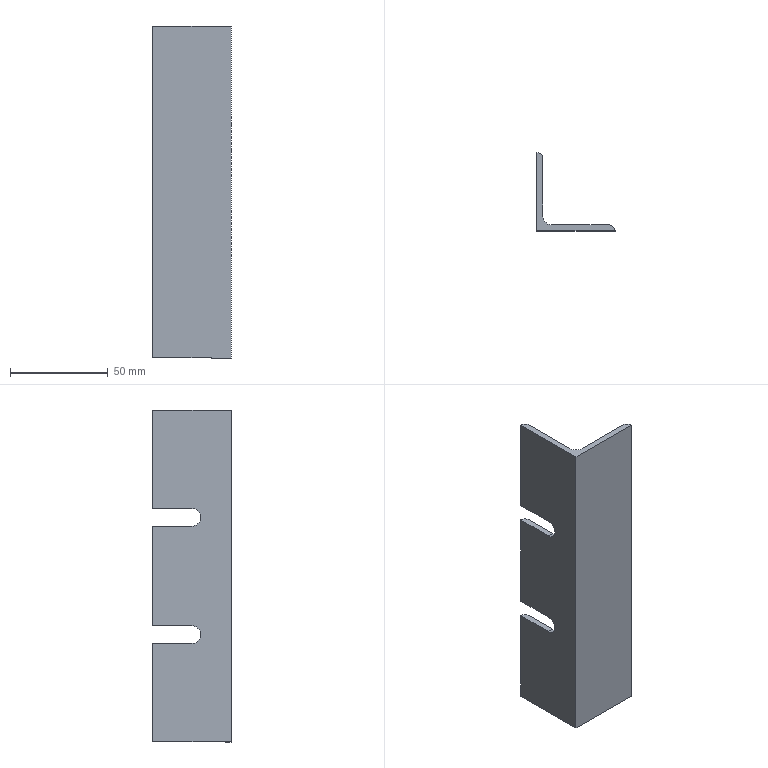Part | SolidWorks | features BaseBody 1 | 1 solid | 17 faces | box 40 x 40 x 170 mm | volume 38116 mm3 | plane 10 | cylinder 7 | commonest cylinder face diameters 6 x4 9 x3
STEP:
#1=CARTESIAN_POINT('',(3.,37.,25.5));
#2=VERTEX_POINT('',#1);
#3=CARTESIAN_POINT('',(0.,40.,25.5));
#4=VERTEX_POINT('',#3);
#5=CARTESIAN_POINT('',(0.,37.,25.5));
#6=DIRECTION('',(0.,0.,1.));
#7=DIRECTION('',(0.,1.,0.));
#8=AXIS2_PLACEMENT_3D('',#5,#6,#7);
#9=CIRCLE('',#8,3.);
#10=EDGE_CURVE('',#2,#4,#9,.T.);
#11=ORIENTED_EDGE('',*,*,#10,.T.);
#12=CARTESIAN_POINT('',(0.,20.,25.5));
#13=VERTEX_POINT('',#12);
#14=CARTESIAN_POINT('',(0.,40.,25.5));
#15=DIRECTION('',(0.,-1.,0.));
#16=VECTOR('',#15,1000.);
#17=LINE('',#14,#16);
#18=EDGE_CURVE('',#4,#13,#17,.T.);
#19=ORIENTED_EDGE('',*,*,#18,.T.);
#20=CARTESIAN_POINT('',(3.,20.,25.5));
#21=VERTEX_POINT('',#20);
#22=CARTESIAN_POINT('',(10.,20.,25.5));
#23=DIRECTION('',(-1.,0.,0.));
#24=VECTOR('',#23,1000.);
#25=LINE('',#22,#24);
#26=EDGE_CURVE('',#21,#13,#25,.T.);
#27=ORIENTED_EDGE('',*,*,#26,.F.);
#28=CARTESIAN_POINT('',(3.,40.,25.5));
#29=DIRECTION('',(0.,-1.,0.));
#30=VECTOR('',#29,1000.);
#31=LINE('',#28,#30);
#32=EDGE_CURVE('',#2,#21,#31,.T.);
#33=ORIENTED_EDGE('',*,*,#32,.F.);
#34=EDGE_LOOP('',(#11,#19,#27,#33));
#35=FACE_OUTER_BOUND('',#34,.T.);
#36=CARTESIAN_POINT('',(10.,40.,25.5));
#37=DIRECTION('',(0.,0.,-1.));
#38=DIRECTION('',(0.,-1.,0.));
#39=AXIS2_PLACEMENT_3D('',#36,#37,#38);
#40=PLANE('',#39);
#41=ADVANCED_FACE('',(#35),#40,.F.);
#42=CARTESIAN_POINT('',(3.,20.,34.5));
#43=VERTEX_POINT('',#42);
#44=CARTESIAN_POINT('',(0.,20.,34.5));
#45=VERTEX_POINT('',#44);
#46=CARTESIAN_POINT('',(10.,20.,34.5));
#47=DIRECTION('',(-1.,0.,0.));
#48=VECTOR('',#47,1000.);
#49=LINE('',#46,#48);
#50=EDGE_CURVE('',#43,#45,#49,.T.);
#51=ORIENTED_EDGE('',*,*,#50,.T.);
#52=CARTESIAN_POINT('',(0.,40.,34.5));
#53=VERTEX_POINT('',#52);
#54=CARTESIAN_POINT('',(0.,40.,34.5));
#55=DIRECTION('',(0.,1.,0.));
#56=VECTOR('',#55,1000.);
#57=LINE('',#54,#56);
#58=EDGE_CURVE('',#45,#53,#57,.T.);
#59=ORIENTED_EDGE('',*,*,#58,.T.);
#60=CARTESIAN_POINT('',(3.,37.,34.5));
#61=VERTEX_POINT('',#60);
#62=CARTESIAN_POINT('',(0.,37.,34.5));
#63=DIRECTION('',(0.,0.,-1.));
#64=DIRECTION('',(0.,-1.,0.));
#65=AXIS2_PLACEMENT_3D('',#62,#63,#64);
#66=CIRCLE('',#65,3.);
#67=EDGE_CURVE('',#53,#61,#66,.T.);
#68=ORIENTED_EDGE('',*,*,#67,.T.);
#69=CARTESIAN_POINT('',(3.,40.,34.5));
#70=DIRECTION('',(0.,1.,0.));
#71=VECTOR('',#70,1000.);
#72=LINE('',#69,#71);
#73=EDGE_CURVE('',#43,#61,#72,.T.);
#74=ORIENTED_EDGE('',*,*,#73,.F.);
#75=EDGE_LOOP('',(#51,#59,#68,#74));
#76=FACE_OUTER_BOUND('',#75,.T.);
#77=CARTESIAN_POINT('',(10.,40.,34.5));
#78=DIRECTION('',(0.,0.,1.));
#79=DIRECTION('',(0.,-1.,0.));
#80=AXIS2_PLACEMENT_3D('',#77,#78,#79);
#81=PLANE('',#80);
#82=ADVANCED_FACE('',(#76),#81,.F.);
#83=ORIENTED_EDGE('',*,*,#26,.T.);
#84=CARTESIAN_POINT('',(0.,20.,30.));
#85=DIRECTION('',(-1.,0.,0.));
#86=DIRECTION('',(0.,0.,1.));
#87=AXIS2_PLACEMENT_3D('',#84,#85,#86);
#88=CIRCLE('',#87,4.5);
#89=EDGE_CURVE('',#13,#45,#88,.T.);
#90=ORIENTED_EDGE('',*,*,#89,.T.);
#91=ORIENTED_EDGE('',*,*,#50,.F.);
#92=CARTESIAN_POINT('',(3.,20.,30.));
#93=DIRECTION('',(-1.,0.,0.));
#94=DIRECTION('',(0.,-1.,0.));
#95=AXIS2_PLACEMENT_3D('',#92,#93,#94);
#96=CIRCLE('',#95,4.5);
#97=EDGE_CURVE('',#21,#43,#96,.T.);
#98=ORIENTED_EDGE('',*,*,#97,.F.);
#99=EDGE_LOOP('',(#83,#90,#91,#98));
#100=FACE_OUTER_BOUND('',#99,.T.);
#101=CARTESIAN_POINT('',(10.,20.,30.));
#102=DIRECTION('',(-1.,0.,0.));
#103=DIRECTION('',(0.,0.,1.));
#104=AXIS2_PLACEMENT_3D('',#101,#102,#103);
#105=CYLINDRICAL_SURFACE('',#104,4.5);
#106=ADVANCED_FACE('',(#100),#105,.F.);
#107=CARTESIAN_POINT('',(3.,37.,-34.5));
#108=VERTEX_POINT('',#107);
#109=CARTESIAN_POINT('',(0.,40.,-34.5));
#110=VERTEX_POINT('',#109);
#111=CARTESIAN_POINT('',(0.,37.,-34.5));
#112=DIRECTION('',(0.,0.,1.));
#113=DIRECTION('',(0.,1.,0.));
#114=AXIS2_PLACEMENT_3D('',#111,#112,#113);
#115=CIRCLE('',#114,3.);
#116=EDGE_CURVE('',#108,#110,#115,.T.);
#117=ORIENTED_EDGE('',*,*,#116,.T.);
#118=CARTESIAN_POINT('',(0.,20.,-34.5));
#119=VERTEX_POINT('',#118);
#120=CARTESIAN_POINT('',(0.,40.,-34.5));
#121=DIRECTION('',(0.,-1.,0.));
#122=VECTOR('',#121,1000.);
#123=LINE('',#120,#122);
#124=EDGE_CURVE('',#110,#119,#123,.T.);
#125=ORIENTED_EDGE('',*,*,#124,.T.);
#126=CARTESIAN_POINT('',(3.,20.,-34.5));
#127=VERTEX_POINT('',#126);
#128=CARTESIAN_POINT('',(10.,20.,-34.5));
#129=DIRECTION('',(-1.,0.,0.));
#130=VECTOR('',#129,1000.);
#131=LINE('',#128,#130);
#132=EDGE_CURVE('',#127,#119,#131,.T.);
#133=ORIENTED_EDGE('',*,*,#132,.F.);
#134=CARTESIAN_POINT('',(3.,40.,-34.5));
#135=DIRECTION('',(0.,-1.,0.));
#136=VECTOR('',#135,1000.);
#137=LINE('',#134,#136);
#138=EDGE_CURVE('',#108,#127,#137,.T.);
#139=ORIENTED_EDGE('',*,*,#138,.F.);
#140=EDGE_LOOP('',(#117,#125,#133,#139));
#141=FACE_OUTER_BOUND('',#140,.T.);
#142=CARTESIAN_POINT('',(10.,40.,-34.5));
#143=DIRECTION('',(0.,0.,-1.));
#144=DIRECTION('',(0.,-1.,0.));
#145=AXIS2_PLACEMENT_3D('',#142,#143,#144);
#146=PLANE('',#145);
#147=ADVANCED_FACE('',(#141),#146,.F.);
#148=CARTESIAN_POINT('',(3.,20.,-25.5));
#149=VERTEX_POINT('',#148);
#150=CARTESIAN_POINT('',(0.,20.,-25.5));
#151=VERTEX_POINT('',#150);
#152=CARTESIAN_POINT('',(10.,20.,-25.5));
#153=DIRECTION('',(-1.,0.,0.));
#154=VECTOR('',#153,1000.);
#155=LINE('',#152,#154);
#156=EDGE_CURVE('',#149,#151,#155,.T.);
#157=ORIENTED_EDGE('',*,*,#156,.T.);
#158=CARTESIAN_POINT('',(0.,40.,-25.5));
#159=VERTEX_POINT('',#158);
#160=CARTESIAN_POINT('',(0.,40.,-25.5));
#161=DIRECTION('',(0.,1.,0.));
#162=VECTOR('',#161,1000.);
#163=LINE('',#160,#162);
#164=EDGE_CURVE('',#151,#159,#163,.T.);
#165=ORIENTED_EDGE('',*,*,#164,.T.);
#166=CARTESIAN_POINT('',(3.,37.,-25.5));
#167=VERTEX_POINT('',#166);
#168=CARTESIAN_POINT('',(0.,37.,-25.5));
#169=DIRECTION('',(0.,0.,-1.));
#170=DIRECTION('',(1.,0.,0.));
#171=AXIS2_PLACEMENT_3D('',#168,#169,#170);
#172=CIRCLE('',#171,3.);
#173=EDGE_CURVE('',#159,#167,#172,.T.);
#174=ORIENTED_EDGE('',*,*,#173,.T.);
#175=CARTESIAN_POINT('',(3.,40.,-25.5));
#176=DIRECTION('',(0.,1.,0.));
#177=VECTOR('',#176,1000.);
#178=LINE('',#175,#177);
#179=EDGE_CURVE('',#149,#167,#178,.T.);
#180=ORIENTED_EDGE('',*,*,#179,.F.);
#181=EDGE_LOOP('',(#157,#165,#174,#180));
#182=FACE_OUTER_BOUND('',#181,.T.);
#183=CARTESIAN_POINT('',(10.,40.,-25.5));
#184=DIRECTION('',(0.,0.,1.));
#185=DIRECTION('',(1.,0.,0.));
#186=AXIS2_PLACEMENT_3D('',#183,#184,#185);
#187=PLANE('',#186);
#188=ADVANCED_FACE('',(#182),#187,.F.);
#189=ORIENTED_EDGE('',*,*,#132,.T.);
#190=CARTESIAN_POINT('',(0.,20.,-30.));
#191=DIRECTION('',(-1.,0.,0.));
#192=DIRECTION('',(0.,0.,-1.));
#193=AXIS2_PLACEMENT_3D('',#190,#191,#192);
#194=CIRCLE('',#193,4.5);
#195=EDGE_CURVE('',#119,#151,#194,.T.);
#196=ORIENTED_EDGE('',*,*,#195,.T.);
#197=ORIENTED_EDGE('',*,*,#156,.F.);
#198=CARTESIAN_POINT('',(3.,20.,-30.));
#199=DIRECTION('',(-1.,0.,0.));
#200=DIRECTION('',(0.,-1.,0.));
#201=AXIS2_PLACEMENT_3D('',#198,#199,#200);
#202=CIRCLE('',#201,4.5);
#203=EDGE_CURVE('',#127,#149,#202,.T.);
#204=ORIENTED_EDGE('',*,*,#203,.F.);
#205=EDGE_LOOP('',(#189,#196,#197,#204));
#206=FACE_OUTER_BOUND('',#205,.T.);
#207=CARTESIAN_POINT('',(10.,20.,-30.));
#208=DIRECTION('',(-1.,0.,0.));
#209=DIRECTION('',(0.,0.,1.));
#210=AXIS2_PLACEMENT_3D('',#207,#208,#209);
#211=CYLINDRICAL_SURFACE('',#210,4.5);
#212=ADVANCED_FACE('',(#206),#211,.F.);
#213=ORIENTED_EDGE('',*,*,#116,.F.);
#214=CARTESIAN_POINT('',(3.,37.,-85.));
#215=VERTEX_POINT('',#214);
#216=CARTESIAN_POINT('',(3.,37.,85.));
#217=DIRECTION('',(0.,0.,1.));
#218=VECTOR('',#217,1000.);
#219=LINE('',#216,#218);
#220=EDGE_CURVE('',#215,#108,#219,.T.);
#221=ORIENTED_EDGE('',*,*,#220,.F.);
#222=CARTESIAN_POINT('',(0.,40.,-85.));
#223=VERTEX_POINT('',#222);
#224=CARTESIAN_POINT('',(0.,37.,-85.));
#225=DIRECTION('',(0.,0.,-1.));
#226=DIRECTION('',(-1.,0.,0.));
#227=AXIS2_PLACEMENT_3D('',#224,#225,#226);
#228=CIRCLE('',#227,3.);
#229=EDGE_CURVE('',#223,#215,#228,.T.);
#230=ORIENTED_EDGE('',*,*,#229,.F.);
#231=CARTESIAN_POINT('',(0.,40.,85.));
#232=DIRECTION('',(0.,0.,-1.));
#233=VECTOR('',#232,1000.);
#234=LINE('',#231,#233);
#235=EDGE_CURVE('',#110,#223,#234,.T.);
#236=ORIENTED_EDGE('',*,*,#235,.F.);
#237=EDGE_LOOP('',(#213,#221,#230,#236));
#238=FACE_OUTER_BOUND('',#237,.T.);
#239=CARTESIAN_POINT('',(0.,37.,85.));
#240=DIRECTION('',(0.,0.,-1.));
#241=DIRECTION('',(-1.,0.,0.));
#242=AXIS2_PLACEMENT_3D('',#239,#240,#241);
#243=CYLINDRICAL_SURFACE('',#242,3.);
#244=ADVANCED_FACE('',(#238),#243,.T.);
#245=CARTESIAN_POINT('',(40.,0.,85.));
#246=VERTEX_POINT('',#245);
#247=CARTESIAN_POINT('',(37.,3.,85.));
#248=VERTEX_POINT('',#247);
#249=CARTESIAN_POINT('',(37.,0.,85.));
#250=DIRECTION('',(0.,0.,1.));
#251=DIRECTION('',(-1.,0.,0.));
#252=AXIS2_PLACEMENT_3D('',#249,#250,#251);
#253=CIRCLE('',#252,3.);
#254=EDGE_CURVE('',#246,#248,#253,.T.);
#255=ORIENTED_EDGE('',*,*,#254,.F.);
#256=CARTESIAN_POINT('',(40.,0.,-85.));
#257=VERTEX_POINT('',#256);
#258=CARTESIAN_POINT('',(40.,0.,85.));
#259=DIRECTION('',(0.,0.,-1.));
#260=VECTOR('',#259,1000.);
#261=LINE('',#258,#260);
#262=EDGE_CURVE('',#246,#257,#261,.T.);
#263=ORIENTED_EDGE('',*,*,#262,.T.);
#264=CARTESIAN_POINT('',(37.,3.,-85.));
#265=VERTEX_POINT('',#264);
#266=CARTESIAN_POINT('',(37.,0.,-85.));
#267=DIRECTION('',(0.,0.,-1.));
#268=DIRECTION('',(-1.,0.,0.));
#269=AXIS2_PLACEMENT_3D('',#266,#267,#268);
#270=CIRCLE('',#269,3.);
#271=EDGE_CURVE('',#265,#257,#270,.T.);
#272=ORIENTED_EDGE('',*,*,#271,.F.);
#273=CARTESIAN_POINT('',(37.,3.,85.));
#274=DIRECTION('',(0.,0.,-1.));
#275=VECTOR('',#274,1000.);
#276=LINE('',#273,#275);
#277=EDGE_CURVE('',#248,#265,#276,.T.);
#278=ORIENTED_EDGE('',*,*,#277,.F.);
#279=EDGE_LOOP('',(#255,#263,#272,#278));
#280=FACE_OUTER_BOUND('',#279,.T.);
#281=CARTESIAN_POINT('',(37.,0.,85.));
#282=DIRECTION('',(0.,0.,-1.));
#283=DIRECTION('',(-1.,0.,0.));
#284=AXIS2_PLACEMENT_3D('',#281,#282,#283);
#285=CYLINDRICAL_SURFACE('',#284,3.);
#286=ADVANCED_FACE('',(#280),#285,.T.);
#287=CARTESIAN_POINT('',(7.5,3.,85.));
#288=VERTEX_POINT('',#287);
#289=CARTESIAN_POINT('',(3.,7.5,85.));
#290=VERTEX_POINT('',#289);
#291=CARTESIAN_POINT('',(7.5,7.5,85.));
#292=DIRECTION('',(0.,0.,-1.));
#293=DIRECTION('',(-1.,0.,0.));
#294=AXIS2_PLACEMENT_3D('',#291,#292,#293);
#295=CIRCLE('',#294,4.5);
#296=EDGE_CURVE('',#288,#290,#295,.T.);
#297=ORIENTED_EDGE('',*,*,#296,.F.);
#298=CARTESIAN_POINT('',(7.5,3.,-85.));
#299=VERTEX_POINT('',#298);
#300=CARTESIAN_POINT('',(7.5,3.,85.));
#301=DIRECTION('',(0.,0.,1.));
#302=VECTOR('',#301,1000.);
#303=LINE('',#300,#302);
#304=EDGE_CURVE('',#299,#288,#303,.T.);
#305=ORIENTED_EDGE('',*,*,#304,.F.);
#306=CARTESIAN_POINT('',(3.,7.5,-85.));
#307=VERTEX_POINT('',#306);
#308=CARTESIAN_POINT('',(7.5,7.5,-85.));
#309=DIRECTION('',(0.,0.,1.));
#310=DIRECTION('',(-1.,0.,0.));
#311=AXIS2_PLACEMENT_3D('',#308,#309,#310);
#312=CIRCLE('',#311,4.5);
#313=EDGE_CURVE('',#307,#299,#312,.T.);
#314=ORIENTED_EDGE('',*,*,#313,.F.);
#315=CARTESIAN_POINT('',(3.,7.5,-85.));
#316=DIRECTION('',(0.,0.,-1.));
#317=VECTOR('',#316,1000.);
#318=LINE('',#315,#317);
#319=EDGE_CURVE('',#290,#307,#318,.T.);
#320=ORIENTED_EDGE('',*,*,#319,.F.);
#321=EDGE_LOOP('',(#297,#305,#314,#320));
#322=FACE_OUTER_BOUND('',#321,.T.);
#323=CARTESIAN_POINT('',(7.5,7.5,85.));
#324=DIRECTION('',(0.,0.,1.));
#325=DIRECTION('',(1.,0.,0.));
#326=AXIS2_PLACEMENT_3D('',#323,#324,#325);
#327=CYLINDRICAL_SURFACE('',#326,4.5);
#328=ADVANCED_FACE('',(#322),#327,.F.);
#329=CARTESIAN_POINT('',(3.,3.,-85.));
#330=DIRECTION('',(-1.,0.,0.));
#331=VECTOR('',#330,1000.);
#332=LINE('',#329,#331);
#333=EDGE_CURVE('',#265,#299,#332,.T.);
#334=ORIENTED_EDGE('',*,*,#333,.F.);
#335=ORIENTED_EDGE('',*,*,#271,.T.);
#336=CARTESIAN_POINT('',(0.,0.,-85.));
#337=VERTEX_POINT('',#336);
#338=CARTESIAN_POINT('',(0.,0.,-85.));
#339=DIRECTION('',(1.,0.,0.));
#340=VECTOR('',#339,1000.);
#341=LINE('',#338,#340);
#342=EDGE_CURVE('',#337,#257,#341,.T.);
#343=ORIENTED_EDGE('',*,*,#342,.F.);
#344=CARTESIAN_POINT('',(0.,0.,-85.));
#345=DIRECTION('',(0.,-1.,0.));
#346=VECTOR('',#345,1000.);
#347=LINE('',#344,#346);
#348=EDGE_CURVE('',#223,#337,#347,.T.);
#349=ORIENTED_EDGE('',*,*,#348,.F.);
#350=ORIENTED_EDGE('',*,*,#229,.T.);
#351=CARTESIAN_POINT('',(3.,40.,-85.));
#352=DIRECTION('',(0.,1.,0.));
#353=VECTOR('',#352,1000.);
#354=LINE('',#351,#353);
#355=EDGE_CURVE('',#307,#215,#354,.T.);
#356=ORIENTED_EDGE('',*,*,#355,.F.);
#357=ORIENTED_EDGE('',*,*,#313,.T.);
#358=EDGE_LOOP('',(#334,#335,#343,#349,#350,#356,#357));
#359=FACE_OUTER_BOUND('',#358,.T.);
#360=CARTESIAN_POINT('',(0.,0.,-85.));
#361=DIRECTION('',(0.,0.,-1.));
#362=DIRECTION('',(0.,-1.,0.));
#363=AXIS2_PLACEMENT_3D('',#360,#361,#362);
#364=PLANE('',#363);
#365=ADVANCED_FACE('',(#359),#364,.T.);
#366=CARTESIAN_POINT('',(0.,0.,85.));
#367=VERTEX_POINT('',#366);
#368=CARTESIAN_POINT('',(0.,0.,85.));
#369=DIRECTION('',(1.,0.,0.));
#370=VECTOR('',#369,1000.);
#371=LINE('',#368,#370);
#372=EDGE_CURVE('',#367,#246,#371,.T.);
#373=ORIENTED_EDGE('',*,*,#372,.T.);
#374=ORIENTED_EDGE('',*,*,#254,.T.);
#375=CARTESIAN_POINT('',(3.,3.,85.));
#376=DIRECTION('',(-1.,0.,0.));
#377=VECTOR('',#376,1000.);
#378=LINE('',#375,#377);
#379=EDGE_CURVE('',#248,#288,#378,.T.);
#380=ORIENTED_EDGE('',*,*,#379,.T.);
#381=ORIENTED_EDGE('',*,*,#296,.T.);
#382=CARTESIAN_POINT('',(3.,37.,85.));
#383=VERTEX_POINT('',#382);
#384=CARTESIAN_POINT('',(3.,40.,85.));
#385=DIRECTION('',(0.,1.,0.));
#386=VECTOR('',#385,1000.);
#387=LINE('',#384,#386);
#388=EDGE_CURVE('',#290,#383,#387,.T.);
#389=ORIENTED_EDGE('',*,*,#388,.T.);
#390=CARTESIAN_POINT('',(0.,40.,85.));
#391=VERTEX_POINT('',#390);
#392=CARTESIAN_POINT('',(0.,37.,85.));
#393=DIRECTION('',(0.,0.,1.));
#394=DIRECTION('',(-1.,0.,0.));
#395=AXIS2_PLACEMENT_3D('',#392,#393,#394);
#396=CIRCLE('',#395,3.);
#397=EDGE_CURVE('',#383,#391,#396,.T.);
#398=ORIENTED_EDGE('',*,*,#397,.T.);
#399=CARTESIAN_POINT('',(0.,0.,85.));
#400=DIRECTION('',(0.,-1.,0.));
#401=VECTOR('',#400,1000.);
#402=LINE('',#399,#401);
#403=EDGE_CURVE('',#391,#367,#402,.T.);
#404=ORIENTED_EDGE('',*,*,#403,.T.);
#405=EDGE_LOOP('',(#373,#374,#380,#381,#389,#398,#404));
#406=FACE_OUTER_BOUND('',#405,.T.);
#407=CARTESIAN_POINT('',(0.,0.,85.));
#408=DIRECTION('',(0.,0.,-1.));
#409=DIRECTION('',(0.,-1.,0.));
#410=AXIS2_PLACEMENT_3D('',#407,#408,#409);
#411=PLANE('',#410);
#412=ADVANCED_FACE('',(#406),#411,.F.);
#413=ORIENTED_EDGE('',*,*,#97,.T.);
#414=ORIENTED_EDGE('',*,*,#73,.T.);
#415=CARTESIAN_POINT('',(3.,37.,85.));
#416=DIRECTION('',(0.,0.,1.));
#417=VECTOR('',#416,1000.);
#418=LINE('',#415,#417);
#419=EDGE_CURVE('',#61,#383,#418,.T.);
#420=ORIENTED_EDGE('',*,*,#419,.T.);
#421=ORIENTED_EDGE('',*,*,#388,.F.);
#422=ORIENTED_EDGE('',*,*,#319,.T.);
#423=ORIENTED_EDGE('',*,*,#355,.T.);
#424=ORIENTED_EDGE('',*,*,#220,.T.);
#425=ORIENTED_EDGE('',*,*,#138,.T.);
#426=ORIENTED_EDGE('',*,*,#203,.T.);
#427=ORIENTED_EDGE('',*,*,#179,.T.);
#428=CARTESIAN_POINT('',(3.,37.,85.));
#429=DIRECTION('',(0.,0.,1.));
#430=VECTOR('',#429,1000.);
#431=LINE('',#428,#430);
#432=EDGE_CURVE('',#167,#2,#431,.T.);
#433=ORIENTED_EDGE('',*,*,#432,.T.);
#434=ORIENTED_EDGE('',*,*,#32,.T.);
#435=EDGE_LOOP('',(#413,#414,#420,#421,#422,#423,#424,#425,#426,#427,#433,#434));
#436=FACE_OUTER_BOUND('',#435,.T.);
#437=CARTESIAN_POINT('',(3.,40.,85.));
#438=DIRECTION('',(-1.,0.,0.));
#439=DIRECTION('',(0.,1.,0.));
#440=AXIS2_PLACEMENT_3D('',#437,#438,#439);
#441=PLANE('',#440);
#442=ADVANCED_FACE('',(#436),#441,.F.);
#443=ORIENTED_EDGE('',*,*,#379,.F.);
#444=ORIENTED_EDGE('',*,*,#277,.T.);
#445=ORIENTED_EDGE('',*,*,#333,.T.);
#446=ORIENTED_EDGE('',*,*,#304,.T.);
#447=EDGE_LOOP('',(#443,#444,#445,#446));
#448=FACE_OUTER_BOUND('',#447,.T.);
#449=CARTESIAN_POINT('',(3.,3.,85.));
#450=DIRECTION('',(0.,-1.,0.));
#451=DIRECTION('',(0.,0.,-1.));
#452=AXIS2_PLACEMENT_3D('',#449,#450,#451);
#453=PLANE('',#452);
#454=ADVANCED_FACE('',(#448),#453,.F.);
#455=ORIENTED_EDGE('',*,*,#342,.T.);
#456=ORIENTED_EDGE('',*,*,#262,.F.);
#457=ORIENTED_EDGE('',*,*,#372,.F.);
#458=CARTESIAN_POINT('',(0.,0.,85.));
#459=DIRECTION('',(0.,0.,-1.));
#460=VECTOR('',#459,1000.);
#461=LINE('',#458,#460);
#462=EDGE_CURVE('',#367,#337,#461,.T.);
#463=ORIENTED_EDGE('',*,*,#462,.T.);
#464=EDGE_LOOP('',(#455,#456,#457,#463));
#465=FACE_OUTER_BOUND('',#464,.T.);
#466=CARTESIAN_POINT('',(0.,0.,85.));
#467=DIRECTION('',(0.,1.,0.));
#468=DIRECTION('',(1.,0.,0.));
#469=AXIS2_PLACEMENT_3D('',#466,#467,#468);
#470=PLANE('',#469);
#471=ADVANCED_FACE('',(#465),#470,.F.);
#472=CARTESIAN_POINT('',(0.,40.,85.));
#473=DIRECTION('',(0.,0.,-1.));
#474=VECTOR('',#473,1000.);
#475=LINE('',#472,#474);
#476=EDGE_CURVE('',#391,#53,#475,.T.);
#477=ORIENTED_EDGE('',*,*,#476,.T.);
#478=ORIENTED_EDGE('',*,*,#58,.F.);
#479=ORIENTED_EDGE('',*,*,#89,.F.);
#480=ORIENTED_EDGE('',*,*,#18,.F.);
#481=CARTESIAN_POINT('',(0.,40.,85.));
#482=DIRECTION('',(0.,0.,-1.));
#483=VECTOR('',#482,1000.);
#484=LINE('',#481,#483);
#485=EDGE_CURVE('',#4,#159,#484,.T.);
#486=ORIENTED_EDGE('',*,*,#485,.T.);
#487=ORIENTED_EDGE('',*,*,#164,.F.);
#488=ORIENTED_EDGE('',*,*,#195,.F.);
#489=ORIENTED_EDGE('',*,*,#124,.F.);
#490=ORIENTED_EDGE('',*,*,#235,.T.);
#491=ORIENTED_EDGE('',*,*,#348,.T.);
#492=ORIENTED_EDGE('',*,*,#462,.F.);
#493=ORIENTED_EDGE('',*,*,#403,.F.);
#494=EDGE_LOOP('',(#477,#478,#479,#480,#486,#487,#488,#489,#490,#491,#492,#493));
#495=FACE_OUTER_BOUND('',#494,.T.);
#496=CARTESIAN_POINT('',(0.,0.,85.));
#497=DIRECTION('',(1.,0.,0.));
#498=DIRECTION('',(0.,1.,0.));
#499=AXIS2_PLACEMENT_3D('',#496,#497,#498);
#500=PLANE('',#499);
#501=ADVANCED_FACE('',(#495),#500,.F.);
#502=ORIENTED_EDGE('',*,*,#10,.F.);
#503=ORIENTED_EDGE('',*,*,#432,.F.);
#504=ORIENTED_EDGE('',*,*,#173,.F.);
#505=ORIENTED_EDGE('',*,*,#485,.F.);
#506=EDGE_LOOP('',(#502,#503,#504,#505));
#507=FACE_OUTER_BOUND('',#506,.T.);
#508=CARTESIAN_POINT('',(0.,37.,85.));
#509=DIRECTION('',(0.,0.,-1.));
#510=DIRECTION('',(-1.,0.,0.));
#511=AXIS2_PLACEMENT_3D('',#508,#509,#510);
#512=CYLINDRICAL_SURFACE('',#511,3.);
#513=ADVANCED_FACE('',(#507),#512,.T.);
#514=ORIENTED_EDGE('',*,*,#67,.F.);
#515=ORIENTED_EDGE('',*,*,#476,.F.);
#516=ORIENTED_EDGE('',*,*,#397,.F.);
#517=ORIENTED_EDGE('',*,*,#419,.F.);
#518=EDGE_LOOP('',(#514,#515,#516,#517));
#519=FACE_OUTER_BOUND('',#518,.T.);
#520=CARTESIAN_POINT('',(0.,37.,85.));
#521=DIRECTION('',(0.,0.,-1.));
#522=DIRECTION('',(-1.,0.,0.));
#523=AXIS2_PLACEMENT_3D('',#520,#521,#522);
#524=CYLINDRICAL_SURFACE('',#523,3.);
#525=ADVANCED_FACE('',(#519),#524,.T.);
#526=CLOSED_SHELL('',(#41,#82,#106,#147,#188,#212,#244,#286,#328,#365,#412,#442,#454,#471,#501,#513,#525));
#527=MANIFOLD_SOLID_BREP('',#526);
#528=CARTESIAN_POINT('',(0.,0.,0.));
#529=DIRECTION('',(0.,0.,1.));
#530=DIRECTION('',(1.,0.,0.));
#531=AXIS2_PLACEMENT_3D('',#528,#529,#530);
#532=(LENGTH_UNIT()NAMED_UNIT(*)SI_UNIT(.MILLI.,.METRE.));
#533=UNCERTAINTY_MEASURE_WITH_UNIT(LENGTH_MEASURE(0.00001),#532,'','');
#534=(NAMED_UNIT(*)PLANE_ANGLE_UNIT()SI_UNIT($,.RADIAN.));
#535=(NAMED_UNIT(*)SI_UNIT($,.STERADIAN.)SOLID_ANGLE_UNIT());
#536=(GEOMETRIC_REPRESENTATION_CONTEXT(3)GLOBAL_UNCERTAINTY_ASSIGNED_CONTEXT((#533))GLOBAL_UNIT_ASSIGNED_CONTEXT((#532,#534,#535))REPRESENTATION_CONTEXT('',''));
#537=ADVANCED_BREP_SHAPE_REPRESENTATION('',(#527,#531),#536);